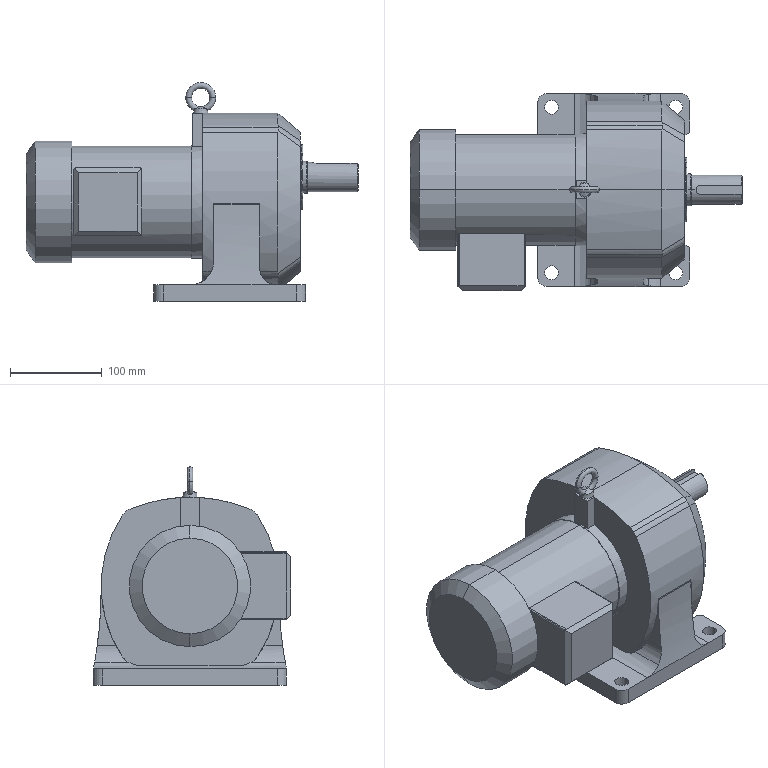Part | STEP file | M2-135-1_2HP-120HT.stp | 1 solid | 137 faces | box 361 x 214.5 x 237.8 mm | volume 6497116 mm3 | cylinder 58 | plane 30 | spline 25 | cone 12 | torus 10 | sphere 2 | commonest cylinder face diameters 40 x12 4 x8 340 x6 15 x4 36 x4 50 x3